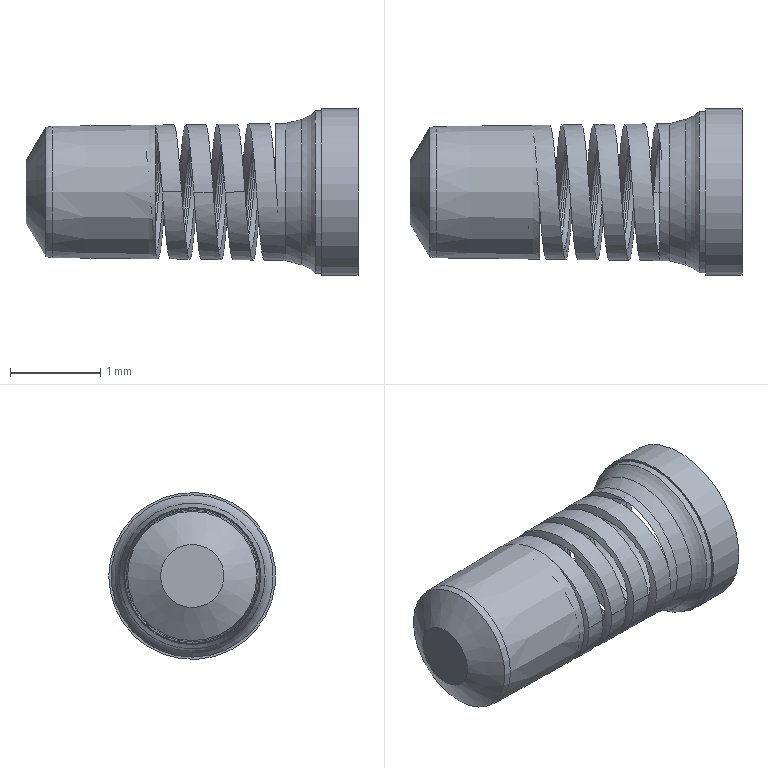Part | STEP file | Basler ace 2 USB3-1-1-1 | 1 solid | 63 faces | box 3.68 x 1.85 x 1.85 mm | volume 2.495 mm3 | spline 34 | cone 13 | cylinder 9 | plane 4 | torus 3 | commonest cylinder face diameters 1.12 x6 1.39 x1 1.8 x1 1.85 x1